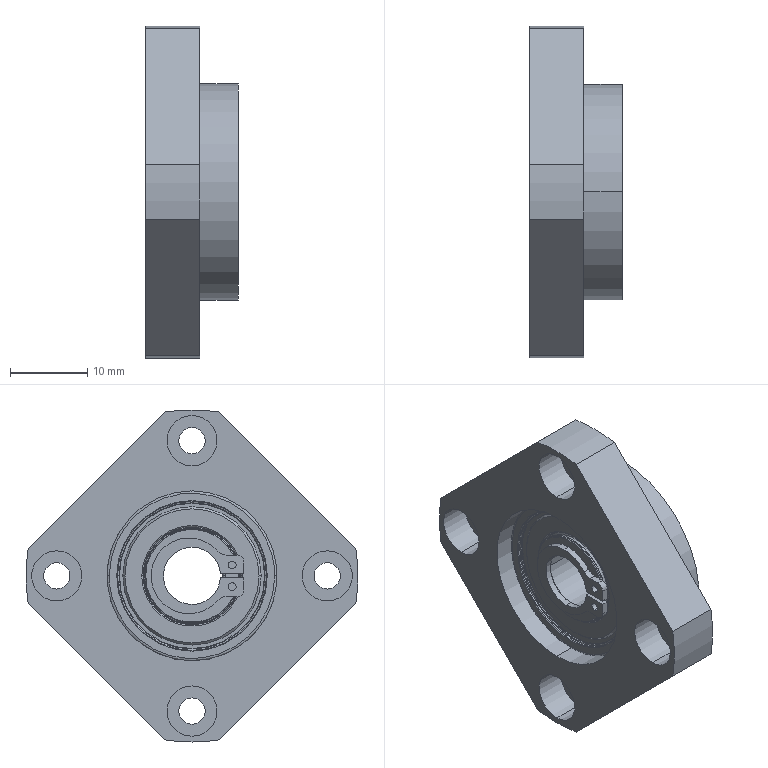Part | SolidWorks | 3 solids | 174 faces | box 12 x 43 x 43 mm | volume 7993 mm3 | cylinder 67 | cone 44 | spline 32 | plane 31 | commonest cylinder face diameters 3.4 x8 6.5 x8 43 x5 1 x4 12.2 x4 12.6 x4